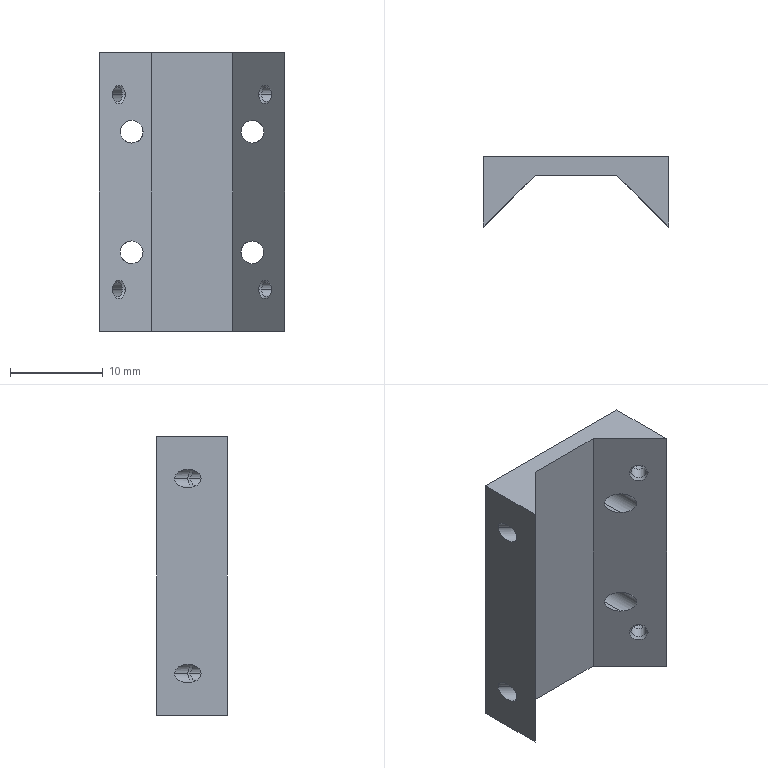Part | STEP file | Guide wheel mechanism revised.sldasm-Part-502 | 1 solid | 56 faces | box 20 x 7.6 x 30 mm | volume 2033 mm3 | cone 24 | cylinder 24 | plane 8 | commonest cylinder face diameters 1.567 x8 2 x8 2.459 x8